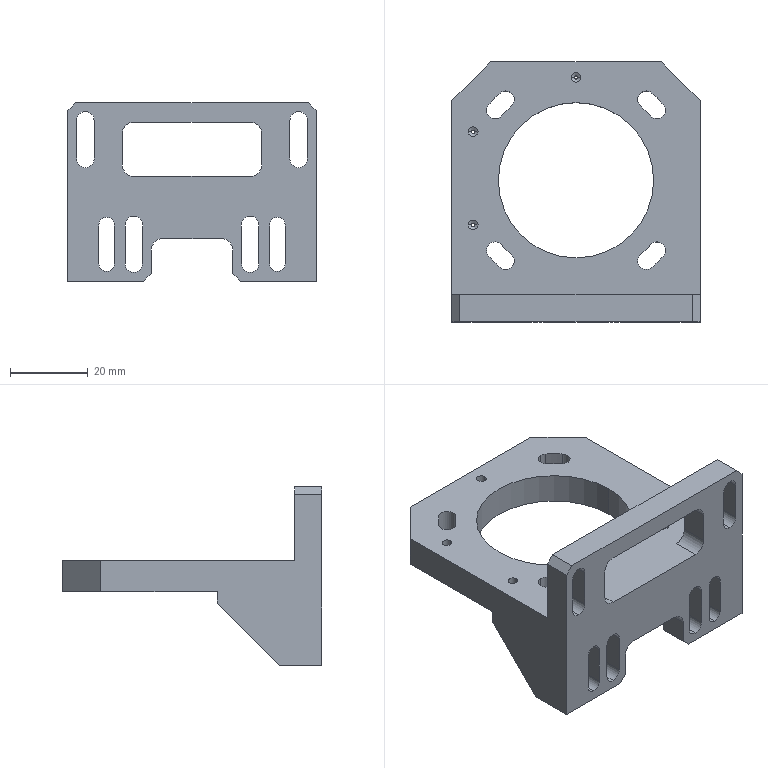NC program | NX | posted with a generic post | part box 64 x 67 x 46 mm
Lines 2506 to 3573 of 8734:
(ZLEVEL_PROFILE_COPY_1_COPY , TOOL : D3)
N4998 T03 M6
N5000 G54
N5002 G17 G0 G90 X-28.2 Y-16.714 B0. C0. S5500 M3
N5004 G43 Z30. H3
N5006 Z0.8
N5008 G94 G1 Y-18.565 Z0.703 F1000.
N5010 X-28.166 Y-18.746 Z0.693
N5012 X-28.017 Y-18.987 Z0.678
N5014 X-27.785 Y-19.15 Z0.664
N5016 X-27.509 Y-19.21 Z0.649
N5018 X-27.231 Y-19.157 Z0.634
N5020 X-27.029 Y-19.031 Z0.622
N5022 X-26.879 Y-18.845 Z0.609
N5024 X-26.8 Y-18.619 Z0.596
N5026 Y-8.381 Z0.06
N5028 X-26.907 Y-8.109 Z0.045
N5030 X-27.115 Y-7.903 Z0.029
N5032 X-27.389 Y-7.799 Z0.014
N5034 X-27.626 Y-7.801 Z0.001
N5036 X-27.893 Y-7.909 Z-0.014
N5038 X-28.095 Y-8.113 Z-0.029
N5040 X-28.2 Y-8.381 Z-0.044
N5042 Y-8.5 Z-0.05
N5044 Y-18.5 F1250.
N5046 G3 X-27.5 Y-19.2 R0.7
N5048 X-26.8 Y-18.5 R0.7
N5050 G1 Y-8.5
N5052 G3 X-27.5 Y-7.8 R0.7
N5054 X-28.2 Y-8.5 R0.7
N5056 G1 Y-11.364 Z-0.1
N5058 Y-18.5
N5060 G3 X-27.5 Y-19.2 R0.7
N5062 X-26.8 Y-18.5 R0.7
N5064 G1 Y-8.5
N5066 G3 X-27.5 Y-7.8 R0.7
N5068 X-28.2 Y-8.5 R0.7
N5070 G1 Y-11.364 Z-0.15
N5072 Y-18.5
N5074 G3 X-27.5 Y-19.2 R0.7
N5076 X-26.8 Y-18.5 R0.7
N5078 G1 Y-8.5
N5080 G3 X-27.5 Y-7.8 R0.7
N5082 X-28.2 Y-8.5 R0.7
N5084 G1 Y-11.364 Z-0.2
N5086 Y-18.5
N5088 G3 X-27.5 Y-19.2 R0.7
N5090 X-26.8 Y-18.5 R0.7
N5092 G1 Y-8.5
N5094 G3 X-27.5 Y-7.8 R0.7
N5096 X-28.2 Y-8.5 R0.7
N5098 G1 Y-11.364 Z-0.25
N5100 Y-18.5
N5102 G3 X-27.5 Y-19.2 R0.7
N5104 X-26.8 Y-18.5 R0.7
N5106 G1 Y-8.5
N5108 G3 X-27.5 Y-7.8 R0.7
N5110 X-28.2 Y-8.5 R0.7
N5112 G1 Y-11.364 Z-0.3
N5114 Y-18.5
N5116 G3 X-27.5 Y-19.2 R0.7
N5118 X-26.8 Y-18.5 R0.7
N5120 G1 Y-8.5
N5122 G3 X-27.5 Y-7.8 R0.7
N5124 X-28.2 Y-8.5 R0.7
N5126 G1 Y-11.364 Z-0.35
N5128 Y-18.5
N5130 G3 X-27.5 Y-19.2 R0.7
N5132 X-26.8 Y-18.5 R0.7
N5134 G1 Y-8.5
N5136 G3 X-27.5 Y-7.8 R0.7
N5138 X-28.2 Y-8.5 R0.7
N5140 G1 Y-11.364 Z-0.4
N5142 Y-18.5
N5144 G3 X-27.5 Y-19.2 R0.7
N5146 X-26.8 Y-18.5 R0.7
N5148 G1 Y-8.5
N5150 G3 X-27.5 Y-7.8 R0.7
N5152 X-28.2 Y-8.5 R0.7
N5154 G1 Y-11.364 Z-0.45
N5156 Y-18.5
N5158 G3 X-27.5 Y-19.2 R0.7
N5160 X-26.8 Y-18.5 R0.7
N5162 G1 Y-8.5
N5164 G3 X-27.5 Y-7.8 R0.7
N5166 X-28.2 Y-8.5 R0.7
N5168 G1 Y-11.364 Z-0.5
N5170 Y-18.5
N5172 G3 X-27.5 Y-19.2 R0.7
N5174 X-26.8 Y-18.5 R0.7
N5176 G1 Y-8.5
N5178 G3 X-27.5 Y-7.8 R0.7
N5180 X-28.2 Y-8.5 R0.7
N5182 G1 Y-11.364 Z-0.55
N5184 Y-18.5
N5186 G3 X-27.5 Y-19.2 R0.7
N5188 X-26.8 Y-18.5 R0.7
N5190 G1 Y-8.5
N5192 G3 X-27.5 Y-7.8 R0.7
N5194 X-28.2 Y-8.5 R0.7
N5196 G1 Y-11.364 Z-0.6
N5198 Y-18.5
N5200 G3 X-27.5 Y-19.2 R0.7
N5202 X-26.8 Y-18.5 R0.7
N5204 G1 Y-8.5
N5206 G3 X-27.5 Y-7.8 R0.7
N5208 X-28.2 Y-8.5 R0.7
N5210 G1 Y-11.364 Z-0.65
N5212 Y-18.5
N5214 G3 X-27.5 Y-19.2 R0.7
N5216 X-26.8 Y-18.5 R0.7
N5218 G1 Y-8.5
N5220 G3 X-27.5 Y-7.8 R0.7
N5222 X-28.2 Y-8.5 R0.7
N5224 G1 Y-11.364 Z-0.7
N5226 Y-18.5
N5228 G3 X-27.5 Y-19.2 R0.7
N5230 X-26.8 Y-18.5 R0.7
N5232 G1 Y-8.5
N5234 G3 X-27.5 Y-7.8 R0.7
N5236 X-28.2 Y-8.5 R0.7
N5238 G1 Y-11.364 Z-0.75
N5240 Y-18.5
N5242 G3 X-27.5 Y-19.2 R0.7
N5244 X-26.8 Y-18.5 R0.7
N5246 G1 Y-8.5
N5248 G3 X-27.5 Y-7.8 R0.7
N5250 X-28.2 Y-8.5 R0.7
N5252 G1 Y-11.364 Z-0.8
N5254 Y-18.5
N5256 G3 X-27.5 Y-19.2 R0.7
N5258 X-26.8 Y-18.5 R0.7
N5260 G1 Y-8.5
N5262 G3 X-27.5 Y-7.8 R0.7
N5264 X-28.2 Y-8.5 R0.7
N5266 G1 Y-11.364 Z-0.85
N5268 Y-18.5
N5270 G3 X-27.5 Y-19.2 R0.7
N5272 X-26.8 Y-18.5 R0.7
N5274 G1 Y-8.5
N5276 G3 X-27.5 Y-7.8 R0.7
N5278 X-28.2 Y-8.5 R0.7
N5280 G1 Y-11.364 Z-0.9
N5282 Y-18.5
N5284 G3 X-27.5 Y-19.2 R0.7
N5286 X-26.8 Y-18.5 R0.7
N5288 G1 Y-8.5
N5290 G3 X-27.5 Y-7.8 R0.7
N5292 X-28.2 Y-8.5 R0.7
N5294 G1 Y-11.364 Z-0.95
N5296 Y-18.5
N5298 G3 X-27.5 Y-19.2 R0.7
N5300 X-26.8 Y-18.5 R0.7
N5302 G1 Y-8.5
N5304 G3 X-27.5 Y-7.8 R0.7
N5306 X-28.2 Y-8.5 R0.7
N5308 G1 Y-11.364 Z-1.
N5310 Y-18.5
N5312 G3 X-27.5 Y-19.2 R0.7
N5314 X-26.8 Y-18.5 R0.7
N5316 G1 Y-8.5
N5318 G3 X-27.5 Y-7.8 R0.7
N5320 X-28.2 Y-8.5 R0.7
N5322 G1 Y-11.364 Z-1.05
N5324 Y-18.5
N5326 G3 X-27.5 Y-19.2 R0.7
N5328 X-26.8 Y-18.5 R0.7
N5330 G1 Y-8.5
N5332 G3 X-27.5 Y-7.8 R0.7
N5334 X-28.2 Y-8.5 R0.7
N5336 G1 Y-11.364 Z-1.1
N5338 Y-18.5
N5340 G3 X-27.5 Y-19.2 R0.7
N5342 X-26.8 Y-18.5 R0.7
N5344 G1 Y-8.5
N5346 G3 X-27.5 Y-7.8 R0.7
N5348 X-28.2 Y-8.5 R0.7
N5350 G1 Y-11.364 Z-1.15
N5352 Y-18.5
N5354 G3 X-27.5 Y-19.2 R0.7
N5356 X-26.8 Y-18.5 R0.7
N5358 G1 Y-8.5
N5360 G3 X-27.5 Y-7.8 R0.7
N5362 X-28.2 Y-8.5 R0.7
N5364 G1 Y-11.364 Z-1.2
N5366 Y-18.5
N5368 G3 X-27.5 Y-19.2 R0.7
N5370 X-26.8 Y-18.5 R0.7
N5372 G1 Y-8.5
N5374 G3 X-27.5 Y-7.8 R0.7
N5376 X-28.2 Y-8.5 R0.7
N5378 G1 Y-11.364 Z-1.25
N5380 Y-18.5
N5382 G3 X-27.5 Y-19.2 R0.7
N5384 X-26.8 Y-18.5 R0.7
N5386 G1 Y-8.5
N5388 G3 X-27.5 Y-7.8 R0.7
N5390 X-28.2 Y-8.5 R0.7
N5392 G1 Y-11.364 Z-1.3
N5394 Y-18.5
N5396 G3 X-27.5 Y-19.2 R0.7
N5398 X-26.8 Y-18.5 R0.7
N5400 G1 Y-8.5
N5402 G3 X-27.5 Y-7.8 R0.7
N5404 X-28.2 Y-8.5 R0.7
N5406 G1 Y-11.364 Z-1.35
N5408 Y-18.5
N5410 G3 X-27.5 Y-19.2 R0.7
N5412 X-26.8 Y-18.5 R0.7
N5414 G1 Y-8.5
N5416 G3 X-27.5 Y-7.8 R0.7
N5418 X-28.2 Y-8.5 R0.7
N5420 G1 Y-11.364 Z-1.4
N5422 Y-18.5
N5424 G3 X-27.5 Y-19.2 R0.7
N5426 X-26.8 Y-18.5 R0.7
N5428 G1 Y-8.5
N5430 G3 X-27.5 Y-7.8 R0.7
N5432 X-28.2 Y-8.5 R0.7
N5434 G1 Y-11.364 Z-1.45
N5436 Y-18.5
N5438 G3 X-27.5 Y-19.2 R0.7
N5440 X-26.8 Y-18.5 R0.7
N5442 G1 Y-8.5
N5444 G3 X-27.5 Y-7.8 R0.7
N5446 X-28.2 Y-8.5 R0.7
N5448 G1 Y-11.364 Z-1.5
N5450 Y-18.5
N5452 G3 X-27.5 Y-19.2 R0.7
N5454 X-26.8 Y-18.5 R0.7
N5456 G1 Y-8.5
N5458 G3 X-27.5 Y-7.8 R0.7
N5460 X-28.2 Y-8.5 R0.7
N5462 G1 Y-11.364 Z-1.55
N5464 Y-18.5
N5466 G3 X-27.5 Y-19.2 R0.7
N5468 X-26.8 Y-18.5 R0.7
N5470 G1 Y-8.5
N5472 G3 X-27.5 Y-7.8 R0.7
N5474 X-28.2 Y-8.5 R0.7
N5476 G1 Y-11.364 Z-1.6
N5478 Y-18.5
N5480 G3 X-27.5 Y-19.2 R0.7
N5482 X-26.8 Y-18.5 R0.7
N5484 G1 Y-8.5
N5486 G3 X-27.5 Y-7.8 R0.7
N5488 X-28.2 Y-8.5 R0.7
N5490 G1 Y-11.364 Z-1.65
N5492 Y-18.5
N5494 G3 X-27.5 Y-19.2 R0.7
N5496 X-26.8 Y-18.5 R0.7
N5498 G1 Y-8.5
N5500 G3 X-27.5 Y-7.8 R0.7
N5502 X-28.2 Y-8.5 R0.7
N5504 G1 Y-11.364 Z-1.7
N5506 Y-18.5
N5508 G3 X-27.5 Y-19.2 R0.7
N5510 X-26.8 Y-18.5 R0.7
N5512 G1 Y-8.5
N5514 G3 X-27.5 Y-7.8 R0.7
N5516 X-28.2 Y-8.5 R0.7
N5518 G1 Y-11.364 Z-1.75
N5520 Y-18.5
N5522 G3 X-27.5 Y-19.2 R0.7
N5524 X-26.8 Y-18.5 R0.7
N5526 G1 Y-8.5
N5528 G3 X-27.5 Y-7.8 R0.7
N5530 X-28.2 Y-8.5 R0.7
N5532 G1 Y-11.364 Z-1.8
N5534 Y-18.5
N5536 G3 X-27.5 Y-19.2 R0.7
N5538 X-26.8 Y-18.5 R0.7
N5540 G1 Y-8.5
N5542 G3 X-27.5 Y-7.8 R0.7
N5544 X-28.2 Y-8.5 R0.7
N5546 G1 Y-11.364 Z-1.85
N5548 Y-18.5
N5550 G3 X-27.5 Y-19.2 R0.7
N5552 X-26.8 Y-18.5 R0.7
N5554 G1 Y-8.5
N5556 G3 X-27.5 Y-7.8 R0.7
N5558 X-28.2 Y-8.5 R0.7
N5560 G1 Y-11.364 Z-1.9
N5562 Y-18.5
N5564 G3 X-27.5 Y-19.2 R0.7
N5566 X-26.8 Y-18.5 R0.7
N5568 G1 Y-8.5
N5570 G3 X-27.5 Y-7.8 R0.7
N5572 X-28.2 Y-8.5 R0.7
N5574 G1 Y-11.364 Z-1.95
N5576 Y-18.5
N5578 G3 X-27.5 Y-19.2 R0.7
N5580 X-26.8 Y-18.5 R0.7
N5582 G1 Y-8.5
N5584 G3 X-27.5 Y-7.8 R0.7
N5586 X-28.2 Y-8.5 R0.7
N5588 G1 Y-11.364 Z-2.
N5590 Y-18.5
N5592 G3 X-27.5 Y-19.2 R0.7
N5594 X-26.8 Y-18.5 R0.7
N5596 G1 Y-8.5
N5598 G3 X-27.5 Y-7.8 R0.7
N5600 X-28.2 Y-8.5 R0.7
N5602 G1 Y-11.364 Z-2.05
N5604 Y-18.5
N5606 G3 X-27.5 Y-19.2 R0.7
N5608 X-26.8 Y-18.5 R0.7
N5610 G1 Y-8.5
N5612 G3 X-27.5 Y-7.8 R0.7
N5614 X-28.2 Y-8.5 R0.7
N5616 G1 Y-11.364 Z-2.1
N5618 Y-18.5
N5620 G3 X-27.5 Y-19.2 R0.7
N5622 X-26.8 Y-18.5 R0.7
N5624 G1 Y-8.5
N5626 G3 X-27.5 Y-7.8 R0.7
N5628 X-28.2 Y-8.5 R0.7
N5630 G1 Y-11.364 Z-2.15
N5632 Y-18.5
N5634 G3 X-27.5 Y-19.2 R0.7
N5636 X-26.8 Y-18.5 R0.7
N5638 G1 Y-8.5
N5640 G3 X-27.5 Y-7.8 R0.7
N5642 X-28.2 Y-8.5 R0.7
N5644 G1 Y-11.364 Z-2.2
N5646 Y-18.5
N5648 G3 X-27.5 Y-19.2 R0.7
N5650 X-26.8 Y-18.5 R0.7
N5652 G1 Y-8.5
N5654 G3 X-27.5 Y-7.8 R0.7
N5656 X-28.2 Y-8.5 R0.7
N5658 G1 Y-11.364 Z-2.25
N5660 Y-18.5
N5662 G3 X-27.5 Y-19.2 R0.7
N5664 X-26.8 Y-18.5 R0.7
N5666 G1 Y-8.5
N5668 G3 X-27.5 Y-7.8 R0.7
N5670 X-28.2 Y-8.5 R0.7
N5672 G1 Y-11.364 Z-2.3
N5674 Y-18.5
N5676 G3 X-27.5 Y-19.2 R0.7
N5678 X-26.8 Y-18.5 R0.7
N5680 G1 Y-8.5
N5682 G3 X-27.5 Y-7.8 R0.7
N5684 X-28.2 Y-8.5 R0.7
N5686 G1 Y-11.364 Z-2.35
N5688 Y-18.5
N5690 G3 X-27.5 Y-19.2 R0.7
N5692 X-26.8 Y-18.5 R0.7
N5694 G1 Y-8.5
N5696 G3 X-27.5 Y-7.8 R0.7
N5698 X-28.2 Y-8.5 R0.7
N5700 G1 Y-11.364 Z-2.4
N5702 Y-18.5
N5704 G3 X-27.5 Y-19.2 R0.7
N5706 X-26.8 Y-18.5 R0.7
N5708 G1 Y-8.5
N5710 G3 X-27.5 Y-7.8 R0.7
N5712 X-28.2 Y-8.5 R0.7
N5714 G1 Y-11.364 Z-2.45
N5716 Y-18.5
N5718 G3 X-27.5 Y-19.2 R0.7
N5720 X-26.8 Y-18.5 R0.7
N5722 G1 Y-8.5
N5724 G3 X-27.5 Y-7.8 R0.7
N5726 X-28.2 Y-8.5 R0.7
N5728 G1 Y-11.364 Z-2.5
N5730 Y-18.5
N5732 G3 X-27.5 Y-19.2 R0.7
N5734 X-26.8 Y-18.5 R0.7
N5736 G1 Y-8.5
N5738 G3 X-27.5 Y-7.8 R0.7
N5740 X-28.2 Y-8.5 R0.7
N5742 G1 Y-11.364 Z-2.55
N5744 Y-18.5
N5746 G3 X-27.5 Y-19.2 R0.7
N5748 X-26.8 Y-18.5 R0.7
N5750 G1 Y-8.5
N5752 G3 X-27.5 Y-7.8 R0.7
N5754 X-28.2 Y-8.5 R0.7
N5756 G1 Y-11.364 Z-2.6
N5758 Y-18.5
N5760 G3 X-27.5 Y-19.2 R0.7
N5762 X-26.8 Y-18.5 R0.7
N5764 G1 Y-8.5
N5766 G3 X-27.5 Y-7.8 R0.7
N5768 X-28.2 Y-8.5 R0.7
N5770 G1 Y-11.364 Z-2.65
N5772 Y-18.5
N5774 G3 X-27.5 Y-19.2 R0.7
N5776 X-26.8 Y-18.5 R0.7
N5778 G1 Y-8.5
N5780 G3 X-27.5 Y-7.8 R0.7
N5782 X-28.2 Y-8.5 R0.7
N5784 G1 Y-11.364 Z-2.7
N5786 Y-18.5
N5788 G3 X-27.5 Y-19.2 R0.7
N5790 X-26.8 Y-18.5 R0.7
N5792 G1 Y-8.5
N5794 G3 X-27.5 Y-7.8 R0.7
N5796 X-28.2 Y-8.5 R0.7
N5798 G1 Y-11.364 Z-2.75
N5800 Y-18.5
N5802 G3 X-27.5 Y-19.2 R0.7
N5804 X-26.8 Y-18.5 R0.7
N5806 G1 Y-8.5
N5808 G3 X-27.5 Y-7.8 R0.7
N5810 X-28.2 Y-8.5 R0.7
N5812 G1 Y-11.364 Z-2.8
N5814 Y-18.5
N5816 G3 X-27.5 Y-19.2 R0.7
N5818 X-26.8 Y-18.5 R0.7
N5820 G1 Y-8.5
N5822 G3 X-27.5 Y-7.8 R0.7
N5824 X-28.2 Y-8.5 R0.7
N5826 G1 Y-11.364 Z-2.85
N5828 Y-18.5
N5830 G3 X-27.5 Y-19.2 R0.7
N5832 X-26.8 Y-18.5 R0.7
N5834 G1 Y-8.5
N5836 G3 X-27.5 Y-7.8 R0.7
N5838 X-28.2 Y-8.5 R0.7
N5840 G1 Y-11.364 Z-2.9
N5842 Y-18.5
N5844 G3 X-27.5 Y-19.2 R0.7
N5846 X-26.8 Y-18.5 R0.7
N5848 G1 Y-8.5
N5850 G3 X-27.5 Y-7.8 R0.7
N5852 X-28.2 Y-8.5 R0.7
N5854 G1 Y-11.364 Z-2.95
N5856 Y-18.5
N5858 G3 X-27.5 Y-19.2 R0.7
N5860 X-26.8 Y-18.5 R0.7
N5862 G1 Y-8.5
N5864 G3 X-27.5 Y-7.8 R0.7
N5866 X-28.2 Y-8.5 R0.7
N5868 G1 Y-11.364 Z-3.
N5870 Y-18.5
N5872 G3 X-27.5 Y-19.2 R0.7
N5874 X-26.8 Y-18.5 R0.7
N5876 G1 Y-8.5
N5878 G3 X-27.5 Y-7.8 R0.7
N5880 X-28.2 Y-8.5 R0.7
N5882 G1 Y-11.364 Z-3.05
N5884 Y-18.5
N5886 G3 X-27.5 Y-19.2 R0.7
N5888 X-26.8 Y-18.5 R0.7
N5890 G1 Y-8.5
N5892 G3 X-27.5 Y-7.8 R0.7
N5894 X-28.2 Y-8.5 R0.7
N5896 G1 Y-11.364 Z-3.1
N5898 Y-18.5
N5900 G3 X-27.5 Y-19.2 R0.7
N5902 X-26.8 Y-18.5 R0.7
N5904 G1 Y-8.5
N5906 G3 X-27.5 Y-7.8 R0.7
N5908 X-28.2 Y-8.5 R0.7
N5910 G1 Y-11.364 Z-3.15
N5912 Y-18.5
N5914 G3 X-27.5 Y-19.2 R0.7
N5916 X-26.8 Y-18.5 R0.7
N5918 G1 Y-8.5
N5920 G3 X-27.5 Y-7.8 R0.7
N5922 X-28.2 Y-8.5 R0.7
N5924 G1 Y-11.364 Z-3.2
N5926 Y-18.5
N5928 G3 X-27.5 Y-19.2 R0.7
N5930 X-26.8 Y-18.5 R0.7
N5932 G1 Y-8.5
N5934 G3 X-27.5 Y-7.8 R0.7
N5936 X-28.2 Y-8.5 R0.7
N5938 G1 Y-11.364 Z-3.25
N5940 Y-18.5
N5942 G3 X-27.5 Y-19.2 R0.7
N5944 X-26.8 Y-18.5 R0.7
N5946 G1 Y-8.5
N5948 G3 X-27.5 Y-7.8 R0.7
N5950 X-28.2 Y-8.5 R0.7
N5952 G1 Y-11.364 Z-3.3
N5954 Y-18.5
N5956 G3 X-27.5 Y-19.2 R0.7
N5958 X-26.8 Y-18.5 R0.7
N5960 G1 Y-8.5
N5962 G3 X-27.5 Y-7.8 R0.7
N5964 X-28.2 Y-8.5 R0.7
N5966 G1 Y-11.364 Z-3.35
N5968 Y-18.5
N5970 G3 X-27.5 Y-19.2 R0.7
N5972 X-26.8 Y-18.5 R0.7
N5974 G1 Y-8.5
N5976 G3 X-27.5 Y-7.8 R0.7
N5978 X-28.2 Y-8.5 R0.7
N5980 G1 Y-11.364 Z-3.4
N5982 Y-18.5
N5984 G3 X-27.5 Y-19.2 R0.7
N5986 X-26.8 Y-18.5 R0.7
N5988 G1 Y-8.5
N5990 G3 X-27.5 Y-7.8 R0.7
N5992 X-28.2 Y-8.5 R0.7
N5994 G1 Y-11.364 Z-3.45
N5996 Y-18.5
N5998 G3 X-27.5 Y-19.2 R0.7
N6000 X-26.8 Y-18.5 R0.7
N6002 G1 Y-8.5
N6004 G3 X-27.5 Y-7.8 R0.7
N6006 X-28.2 Y-8.5 R0.7
N6008 G1 Y-11.364 Z-3.5
N6010 Y-18.5
N6012 G3 X-27.5 Y-19.2 R0.7
N6014 X-26.8 Y-18.5 R0.7
N6016 G1 Y-8.5
N6018 G3 X-27.5 Y-7.8 R0.7
N6020 X-28.2 Y-8.5 R0.7
N6022 G1 Y-11.364 Z-3.55
N6024 Y-18.5
N6026 G3 X-27.5 Y-19.2 R0.7
N6028 X-26.8 Y-18.5 R0.7
N6030 G1 Y-8.5
N6032 G3 X-27.5 Y-7.8 R0.7
N6034 X-28.2 Y-8.5 R0.7
N6036 G1 Y-11.364 Z-3.6
N6038 Y-18.5
N6040 G3 X-27.5 Y-19.2 R0.7
N6042 X-26.8 Y-18.5 R0.7
N6044 G1 Y-8.5
N6046 G3 X-27.5 Y-7.8 R0.7
N6048 X-28.2 Y-8.5 R0.7
N6050 G1 Y-11.364 Z-3.65
N6052 Y-18.5
N6054 G3 X-27.5 Y-19.2 R0.7
N6056 X-26.8 Y-18.5 R0.7
N6058 G1 Y-8.5
N6060 G3 X-27.5 Y-7.8 R0.7
N6062 X-28.2 Y-8.5 R0.7
N6064 G1 Y-11.364 Z-3.7
N6066 Y-18.5
N6068 G3 X-27.5 Y-19.2 R0.7
N6070 X-26.8 Y-18.5 R0.7
N6072 G1 Y-8.5
N6074 G3 X-27.5 Y-7.8 R0.7
N6076 X-28.2 Y-8.5 R0.7
N6078 G1 Y-11.364 Z-3.75
N6080 Y-18.5
N6082 G3 X-27.5 Y-19.2 R0.7
N6084 X-26.8 Y-18.5 R0.7
N6086 G1 Y-8.5
N6088 G3 X-27.5 Y-7.8 R0.7
N6090 X-28.2 Y-8.5 R0.7
N6092 G1 Y-11.364 Z-3.8
N6094 Y-18.5
N6096 G3 X-27.5 Y-19.2 R0.7
N6098 X-26.8 Y-18.5 R0.7
N6100 G1 Y-8.5
N6102 G3 X-27.5 Y-7.8 R0.7
N6104 X-28.2 Y-8.5 R0.7
N6106 G1 Y-11.364 Z-3.85
N6108 Y-18.5
N6110 G3 X-27.5 Y-19.2 R0.7
N6112 X-26.8 Y-18.5 R0.7
N6114 G1 Y-8.5
N6116 G3 X-27.5 Y-7.8 R0.7
N6118 X-28.2 Y-8.5 R0.7
N6120 G1 Y-11.364 Z-3.9
N6122 Y-18.5
N6124 G3 X-27.5 Y-19.2 R0.7
N6126 X-26.8 Y-18.5 R0.7
N6128 G1 Y-8.5
N6130 G3 X-27.5 Y-7.8 R0.7
N6132 X-28.2 Y-8.5 R0.7
N6134 G1 Y-11.364 Z-3.95
N6136 Y-18.5
N6138 G3 X-27.5 Y-19.2 R0.7
N6140 X-26.8 Y-18.5 R0.7
N6142 G1 Y-8.5
N6144 G3 X-27.5 Y-7.8 R0.7
N6146 X-28.2 Y-8.5 R0.7
N6148 G1 Y-11.364 Z-4.
N6150 Y-18.5
N6152 G3 X-27.5 Y-19.2 R0.7
N6154 X-26.8 Y-18.5 R0.7
N6156 G1 Y-8.5
N6158 G3 X-27.5 Y-7.8 R0.7
N6160 X-28.2 Y-8.5 R0.7
N6162 G1 Y-11.364 Z-4.05
N6164 Y-18.5
N6166 G3 X-27.5 Y-19.2 R0.7
N6168 X-26.8 Y-18.5 R0.7
N6170 G1 Y-8.5
N6172 G3 X-27.5 Y-7.8 R0.7
N6174 X-28.2 Y-8.5 R0.7
N6176 G1 Y-11.364 Z-4.1
N6178 Y-18.5
N6180 G3 X-27.5 Y-19.2 R0.7
N6182 X-26.8 Y-18.5 R0.7
N6184 G1 Y-8.5
N6186 G3 X-27.5 Y-7.8 R0.7
N6188 X-28.2 Y-8.5 R0.7
N6190 G1 Y-11.364 Z-4.15
N6192 Y-18.5
N6194 G3 X-27.5 Y-19.2 R0.7
N6196 X-26.8 Y-18.5 R0.7
N6198 G1 Y-8.5
N6200 G3 X-27.5 Y-7.8 R0.7
N6202 X-28.2 Y-8.5 R0.7
N6204 G1 Y-11.364 Z-4.2
N6206 Y-18.5
N6208 G3 X-27.5 Y-19.2 R0.7
N6210 X-26.8 Y-18.5 R0.7
N6212 G1 Y-8.5
N6214 G3 X-27.5 Y-7.8 R0.7
N6216 X-28.2 Y-8.5 R0.7
N6218 G1 Y-11.364 Z-4.25
N6220 Y-18.5
N6222 G3 X-27.5 Y-19.2 R0.7
N6224 X-26.8 Y-18.5 R0.7
N6226 G1 Y-8.5
N6228 G3 X-27.5 Y-7.8 R0.7
N6230 X-28.2 Y-8.5 R0.7
N6232 G1 Y-11.364 Z-4.3
N6234 Y-18.5
N6236 G3 X-27.5 Y-19.2 R0.7
N6238 X-26.8 Y-18.5 R0.7
N6240 G1 Y-8.5
N6242 G3 X-27.5 Y-7.8 R0.7
N6244 X-28.2 Y-8.5 R0.7
N6246 G1 Y-11.364 Z-4.35
N6248 Y-18.5
N6250 G3 X-27.5 Y-19.2 R0.7
N6252 X-26.8 Y-18.5 R0.7
N6254 G1 Y-8.5
N6256 G3 X-27.5 Y-7.8 R0.7
N6258 X-28.2 Y-8.5 R0.7
N6260 G1 Y-11.364 Z-4.4
N6262 Y-18.5
N6264 G3 X-27.5 Y-19.2 R0.7
N6266 X-26.8 Y-18.5 R0.7
N6268 G1 Y-8.5
N6270 G3 X-27.5 Y-7.8 R0.7
N6272 X-28.2 Y-8.5 R0.7
N6274 G1 Y-11.364 Z-4.45
N6276 Y-18.5
N6278 G3 X-27.5 Y-19.2 R0.7
N6280 X-26.8 Y-18.5 R0.7
N6282 G1 Y-8.5
N6284 G3 X-27.5 Y-7.8 R0.7
N6286 X-28.2 Y-8.5 R0.7
N6288 G1 Y-11.364 Z-4.5
N6290 Y-18.5
N6292 G3 X-27.5 Y-19.2 R0.7
N6294 X-26.8 Y-18.5 R0.7
N6296 G1 Y-8.5
N6298 G3 X-27.5 Y-7.8 R0.7
N6300 X-28.2 Y-8.5 R0.7
N6302 G1 Y-11.364 Z-4.55
N6304 Y-18.5
N6306 G3 X-27.5 Y-19.2 R0.7
N6308 X-26.8 Y-18.5 R0.7
N6310 G1 Y-8.5
N6312 G3 X-27.5 Y-7.8 R0.7
N6314 X-28.2 Y-8.5 R0.7
N6316 G1 Y-11.364 Z-4.6
N6318 Y-18.5
N6320 G3 X-27.5 Y-19.2 R0.7
N6322 X-26.8 Y-18.5 R0.7
N6324 G1 Y-8.5
N6326 G3 X-27.5 Y-7.8 R0.7
N6328 X-28.2 Y-8.5 R0.7
N6330 G1 Y-11.364 Z-4.65
N6332 Y-18.5
N6334 G3 X-27.5 Y-19.2 R0.7
N6336 X-26.8 Y-18.5 R0.7
N6338 G1 Y-8.5
N6340 G3 X-27.5 Y-7.8 R0.7
N6342 X-28.2 Y-8.5 R0.7
N6344 G1 Y-11.364 Z-4.7
N6346 Y-18.5
N6348 G3 X-27.5 Y-19.2 R0.7
N6350 X-26.8 Y-18.5 R0.7
N6352 G1 Y-8.5
N6354 G3 X-27.5 Y-7.8 R0.7
N6356 X-28.2 Y-8.5 R0.7
N6358 G1 Y-11.364 Z-4.75
N6360 Y-18.5
N6362 G3 X-27.5 Y-19.2 R0.7
N6364 X-26.8 Y-18.5 R0.7
N6366 G1 Y-8.5
N6368 G3 X-27.5 Y-7.8 R0.7
N6370 X-28.2 Y-8.5 R0.7
N6372 G1 Y-11.364 Z-4.8
N6374 Y-18.5
N6376 G3 X-27.5 Y-19.2 R0.7
N6378 X-26.8 Y-18.5 R0.7
N6380 G1 Y-8.5
N6382 G3 X-27.5 Y-7.8 R0.7
N6384 X-28.2 Y-8.5 R0.7
N6386 G1 Y-11.364 Z-4.85
N6388 Y-18.5
N6390 G3 X-27.5 Y-19.2 R0.7
N6392 X-26.8 Y-18.5 R0.7
N6394 G1 Y-8.5
N6396 G3 X-27.5 Y-7.8 R0.7
N6398 X-28.2 Y-8.5 R0.7
N6400 G1 Y-11.364 Z-4.9
N6402 Y-18.5
N6404 G3 X-27.5 Y-19.2 R0.7
N6406 X-26.8 Y-18.5 R0.7
N6408 G1 Y-8.5
N6410 G3 X-27.5 Y-7.8 R0.7
N6412 X-28.2 Y-8.5 R0.7
N6414 G1 Y-11.364 Z-4.95
N6416 Y-18.5
N6418 G3 X-27.5 Y-19.2 R0.7
N6420 X-26.8 Y-18.5 R0.7
N6422 G1 Y-8.5
N6424 G3 X-27.5 Y-7.8 R0.7
N6426 X-28.2 Y-8.5 R0.7
N6428 G1 Y-11.364 Z-5.
N6430 Y-18.5
N6432 G3 X-27.5 Y-19.2 R0.7
N6434 X-26.8 Y-18.5 R0.7
N6436 G1 Y-8.5
N6438 G3 X-27.5 Y-7.8 R0.7
N6440 X-28.2 Y-8.5 R0.7
N6442 G1 Y-11.364 Z-5.05
N6444 Y-18.5
N6446 G3 X-27.5 Y-19.2 R0.7
N6448 X-26.8 Y-18.5 R0.7
N6450 G1 Y-8.5
N6452 G3 X-27.5 Y-7.8 R0.7
N6454 X-28.2 Y-8.5 R0.7
N6456 G1 Y-11.364 Z-5.1
N6458 Y-18.5
N6460 G3 X-27.5 Y-19.2 R0.7
N6462 X-26.8 Y-18.5 R0.7
N6464 G1 Y-8.5
N6466 G3 X-27.5 Y-7.8 R0.7
N6468 X-28.2 Y-8.5 R0.7
N6470 G1 Y-11.364 Z-5.15
N6472 Y-18.5
N6474 G3 X-27.5 Y-19.2 R0.7
N6476 X-26.8 Y-18.5 R0.7
N6478 G1 Y-8.5
N6480 G3 X-27.5 Y-7.8 R0.7
N6482 X-28.2 Y-8.5 R0.7
N6484 G1 Y-11.364 Z-5.2
N6486 Y-18.5
N6488 G3 X-27.5 Y-19.2 R0.7
N6490 X-26.8 Y-18.5 R0.7
N6492 G1 Y-8.5
N6494 G3 X-27.5 Y-7.8 R0.7
N6496 X-28.2 Y-8.5 R0.7
N6498 G1 Y-11.364 Z-5.25
N6500 Y-18.5
N6502 G3 X-27.5 Y-19.2 R0.7
N6504 X-26.8 Y-18.5 R0.7
N6506 G1 Y-8.5
N6508 G3 X-27.5 Y-7.8 R0.7
N6510 X-28.2 Y-8.5 R0.7
N6512 G1 Y-11.364 Z-5.3
N6514 Y-18.5
N6516 G3 X-27.5 Y-19.2 R0.7
N6518 X-26.8 Y-18.5 R0.7
N6520 G1 Y-8.5
N6522 G3 X-27.5 Y-7.8 R0.7
N6524 X-28.2 Y-8.5 R0.7
N6526 G1 Y-11.364 Z-5.35
N6528 Y-18.5
N6530 G3 X-27.5 Y-19.2 R0.7
N6532 X-26.8 Y-18.5 R0.7
N6534 G1 Y-8.5
N6536 G3 X-27.5 Y-7.8 R0.7
N6538 X-28.2 Y-8.5 R0.7
N6540 G1 Y-11.364 Z-5.4
N6542 Y-18.5
N6544 G3 X-27.5 Y-19.2 R0.7
N6546 X-26.8 Y-18.5 R0.7
N6548 G1 Y-8.5
N6550 G3 X-27.5 Y-7.8 R0.7
N6552 X-28.2 Y-8.5 R0.7
N6554 G1 Y-11.364 Z-5.45
N6556 Y-18.5
N6558 G3 X-27.5 Y-19.2 R0.7
N6560 X-26.8 Y-18.5 R0.7
N6562 G1 Y-8.5
N6564 G3 X-27.5 Y-7.8 R0.7
N6566 X-28.2 Y-8.5 R0.7
N6568 G1 Y-11.364 Z-5.5
N6570 Y-18.5
N6572 G3 X-27.5 Y-19.2 R0.7
N6574 X-26.8 Y-18.5 R0.7
N6576 G1 Y-8.5
N6578 G3 X-27.5 Y-7.8 R0.7
N6580 X-28.2 Y-8.5 R0.7
N6582 G1 Y-11.364 Z-5.55
N6584 Y-18.5
N6586 G3 X-27.5 Y-19.2 R0.7
N6588 X-26.8 Y-18.5 R0.7
N6590 G1 Y-8.5
N6592 G3 X-27.5 Y-7.8 R0.7
N6594 X-28.2 Y-8.5 R0.7
N6596 G1 Y-11.364 Z-5.6
N6598 Y-18.5
N6600 G3 X-27.5 Y-19.2 R0.7
N6602 X-26.8 Y-18.5 R0.7
N6604 G1 Y-8.5
N6606 G3 X-27.5 Y-7.8 R0.7
N6608 X-28.2 Y-8.5 R0.7
N6610 G1 Y-11.364 Z-5.65
N6612 Y-18.5
N6614 G3 X-27.5 Y-19.2 R0.7
N6616 X-26.8 Y-18.5 R0.7
N6618 G1 Y-8.5
N6620 G3 X-27.5 Y-7.8 R0.7
N6622 X-28.2 Y-8.5 R0.7
N6624 G1 Y-11.364 Z-5.7
N6626 Y-18.5
N6628 G3 X-27.5 Y-19.2 R0.7
N6630 X-26.8 Y-18.5 R0.7
N6632 G1 Y-8.5
N6634 G3 X-27.5 Y-7.8 R0.7
N6636 X-28.2 Y-8.5 R0.7
N6638 G1 Y-11.364 Z-5.75
N6640 Y-18.5
N6642 G3 X-27.5 Y-19.2 R0.7
N6644 X-26.8 Y-18.5 R0.7
N6646 G1 Y-8.5
N6648 G3 X-27.5 Y-7.8 R0.7
N6650 X-28.2 Y-8.5 R0.7
N6652 G1 Y-11.364 Z-5.8
N6654 Y-18.5
N6656 G3 X-27.5 Y-19.2 R0.7
N6658 X-26.8 Y-18.5 R0.7
N6660 G1 Y-8.5
N6662 G3 X-27.5 Y-7.8 R0.7
N6664 X-28.2 Y-8.5 R0.7
N6666 G1 Y-11.364 Z-5.85
N6668 Y-18.5
N6670 G3 X-27.5 Y-19.2 R0.7
N6672 X-26.8 Y-18.5 R0.7
N6674 G1 Y-8.5
N6676 G3 X-27.5 Y-7.8 R0.7
N6678 X-28.2 Y-8.5 R0.7
N6680 G1 Y-11.364 Z-5.9
N6682 Y-18.5
N6684 G3 X-27.5 Y-19.2 R0.7
N6686 X-26.8 Y-18.5 R0.7
N6688 G1 Y-8.5
N6690 G3 X-27.5 Y-7.8 R0.7
N6692 X-28.2 Y-8.5 R0.7
N6694 G1 Y-11.364 Z-5.95
N6696 Y-18.5
N6698 G3 X-27.5 Y-19.2 R0.7
N6700 X-26.8 Y-18.5 R0.7
N6702 G1 Y-8.5
N6704 G3 X-27.5 Y-7.8 R0.7
N6706 X-28.2 Y-8.5 R0.7
N6708 G1 Y-11.364 Z-6.
N6710 Y-18.5
N6712 G3 X-27.5 Y-19.2 R0.7
N6714 X-26.8 Y-18.5 R0.7
N6716 G1 Y-8.5
N6718 G3 X-27.5 Y-7.8 R0.7
N6720 X-28.2 Y-8.5 R0.7
N6722 G1 Y-11.364 Z-6.05
N6724 Y-18.5
N6726 G3 X-27.5 Y-19.2 R0.7
N6728 X-26.8 Y-18.5 R0.7
N6730 G1 Y-8.5
N6732 G3 X-27.5 Y-7.8 R0.7
N6734 X-28.2 Y-8.5 R0.7
N6736 G1 Y-11.364 Z-6.1
N6738 Y-18.5
N6740 G3 X-27.5 Y-19.2 R0.7
N6742 X-26.8 Y-18.5 R0.7
N6744 G1 Y-8.5
N6746 G3 X-27.5 Y-7.8 R0.7
N6748 X-28.2 Y-8.5 R0.7
N6750 G1 Y-11.364 Z-6.15
N6752 Y-18.5
N6754 G3 X-27.5 Y-19.2 R0.7
N6756 X-26.8 Y-18.5 R0.7
N6758 G1 Y-8.5
N6760 G3 X-27.5 Y-7.8 R0.7
N6762 X-28.2 Y-8.5 R0.7
N6764 G1 Y-11.364 Z-6.2
N6766 Y-18.5
N6768 G3 X-27.5 Y-19.2 R0.7
N6770 X-26.8 Y-18.5 R0.7
N6772 G1 Y-8.5
N6774 G3 X-27.5 Y-7.8 R0.7
N6776 X-28.2 Y-8.5 R0.7
N6778 G1 Y-11.364 Z-6.25
N6780 Y-18.5
N6782 G3 X-27.5 Y-19.2 R0.7
N6784 X-26.8 Y-18.5 R0.7
N6786 G1 Y-8.5
N6788 G3 X-27.5 Y-7.8 R0.7
N6790 X-28.2 Y-8.5 R0.7
N6792 G1 Y-11.364 Z-6.3
N6794 Y-18.5
N6796 G3 X-27.5 Y-19.2 R0.7
N6798 X-26.8 Y-18.5 R0.7
N6800 G1 Y-8.5
N6802 G3 X-27.5 Y-7.8 R0.7
N6804 X-28.2 Y-8.5 R0.7
N6806 G1 Y-11.364 Z-6.35
N6808 Y-18.5
N6810 G3 X-27.5 Y-19.2 R0.7
N6812 X-26.8 Y-18.5 R0.7
N6814 G1 Y-8.5
N6816 G3 X-27.5 Y-7.8 R0.7
N6818 X-28.2 Y-8.5 R0.7
N6820 G1 Y-11.364 Z-6.4
N6822 Y-18.5
N6824 G3 X-27.5 Y-19.2 R0.7
N6826 X-26.8 Y-18.5 R0.7
N6828 G1 Y-8.5
N6830 G3 X-27.5 Y-7.8 R0.7
N6832 X-28.2 Y-8.5 R0.7
N6834 G1 Y-11.364 Z-6.45
N6836 Y-18.5
N6838 G3 X-27.5 Y-19.2 R0.7
N6840 X-26.8 Y-18.5 R0.7
N6842 G1 Y-8.5
N6844 G3 X-27.5 Y-7.8 R0.7
N6846 X-28.2 Y-8.5 R0.7
N6848 G1 Y-11.364 Z-6.5
N6850 Y-18.5
N6852 G3 X-27.5 Y-19.2 R0.7
N6854 X-26.8 Y-18.5 R0.7
N6856 G1 Y-8.5
N6858 G3 X-27.5 Y-7.8 R0.7
N6860 X-28.2 Y-8.5 R0.7
N6862 G1 Y-11.364 Z-6.55
N6864 Y-18.5
N6866 G3 X-27.5 Y-19.2 R0.7
N6868 X-26.8 Y-18.5 R0.7
N6870 G1 Y-8.5
N6872 G3 X-27.5 Y-7.8 R0.7
N6874 X-28.2 Y-8.5 R0.7
N6876 G1 Y-11.364 Z-6.6
N6878 Y-18.5
N6880 G3 X-27.5 Y-19.2 R0.7
N6882 X-26.8 Y-18.5 R0.7
N6884 G1 Y-8.5
N6886 G3 X-27.5 Y-7.8 R0.7
N6888 X-28.2 Y-8.5 R0.7
N6890 G1 Y-11.364 Z-6.65
N6892 Y-18.5
N6894 G3 X-27.5 Y-19.2 R0.7
N6896 X-26.8 Y-18.5 R0.7
N6898 G1 Y-8.5
N6900 G3 X-27.5 Y-7.8 R0.7
N6902 X-28.2 Y-8.5 R0.7
N6904 G1 Y-11.364 Z-6.7
N6906 Y-18.5
N6908 G3 X-27.5 Y-19.2 R0.7
N6910 X-26.8 Y-18.5 R0.7
N6912 G1 Y-8.5
N6914 G3 X-27.5 Y-7.8 R0.7
N6916 X-28.2 Y-8.5 R0.7
N6918 G1 Y-11.364 Z-6.75
N6920 Y-18.5
N6922 G3 X-27.5 Y-19.2 R0.7
N6924 X-26.8 Y-18.5 R0.7
N6926 G1 Y-8.5
N6928 G3 X-27.5 Y-7.8 R0.7
N6930 X-28.2 Y-8.5 R0.7
N6932 G1 Y-11.364 Z-6.8
N6934 Y-18.5
N6936 G3 X-27.5 Y-19.2 R0.7
N6938 X-26.8 Y-18.5 R0.7
N6940 G1 Y-8.5
N6942 G3 X-27.5 Y-7.8 R0.7
N6944 X-28.2 Y-8.5 R0.7
N6946 G1 Y-11.364 Z-6.85
N6948 Y-18.5
N6950 G3 X-27.5 Y-19.2 R0.7
N6952 X-26.8 Y-18.5 R0.7
N6954 G1 Y-8.5
N6956 G3 X-27.5 Y-7.8 R0.7
N6958 X-28.2 Y-8.5 R0.7
N6960 G1 Y-11.364 Z-6.9
N6962 Y-18.5
N6964 G3 X-27.5 Y-19.2 R0.7
N6966 X-26.8 Y-18.5 R0.7
N6968 G1 Y-8.5
N6970 G3 X-27.5 Y-7.8 R0.7
N6972 X-28.2 Y-8.5 R0.7
N6974 G1 Y-11.364 Z-6.95
N6976 Y-18.5
N6978 G3 X-27.5 Y-19.2 R0.7
N6980 X-26.8 Y-18.5 R0.7
N6982 G1 Y-8.5
N6984 G3 X-27.5 Y-7.8 R0.7
N6986 X-28.2 Y-8.5 R0.7
N6988 G1 Y-11.364 Z-7.
N6990 Y-18.5
N6992 G3 X-27.5 Y-19.2 R0.7
N6994 X-26.8 Y-18.5 R0.7
N6996 G1 Y-8.5
N6998 G3 X-27.5 Y-7.8 R0.7
N7000 X-28.2 Y-8.5 R0.7
N7002 G1 Y-11.364
N7004 Z-6.2
N7006 G0 Z30.
N7008 X-15.7 Y10.286
N7010 Z0.8
N7012 G1 Y8.435 Z0.703 F1000.
N7014 X-15.666 Y8.254 Z0.693
N7016 X-15.514 Y8.01 Z0.678
N7018 X-15.278 Y7.847 Z0.663
N7020 X-14.996 Y7.79 Z0.648
N7022 X-14.715 Y7.85 Z0.633
N7024 X-14.516 Y7.98 Z0.621
N7026 X-14.375 Y8.163 Z0.609
N7028 X-14.3 Y8.381 Z0.596
N7030 Y18.619 Z0.06
N7032 X-14.405 Y18.887 Z0.045
N7034 X-14.607 Y19.091 Z0.03
N7036 X-14.874 Y19.199 Z0.015
N7038 X-15.112 Y19.201 Z0.002
N7040 X-15.385 Y19.097 Z-0.013
N7042 X-15.593 Y18.891 Z-0.028
N7044 X-15.7 Y18.619 Z-0.044
N7046 Y18.5 Z-0.05
N7048 Y8.5 F1250.
N7050 G3 X-15. Y7.8 R0.7
N7052 X-14.3 Y8.5 R0.7
N7054 G1 Y18.5
N7056 G3 X-15. Y19.2 R0.7
N7058 X-15.7 Y18.5 R0.7
N7060 G1 Y15.636 Z-0.1
N7062 Y8.5
N7064 G3 X-15. Y7.8 R0.7
N7066 X-14.3 Y8.5 R0.7
N7068 G1 Y18.5
N7070 G3 X-15. Y19.2 R0.7
N7072 X-15.7 Y18.5 R0.7
N7074 G1 Y15.636 Z-0.15
N7076 Y8.5
N7078 G3 X-15. Y7.8 R0.7
N7080 X-14.3 Y8.5 R0.7
N7082 G1 Y18.5
N7084 G3 X-15. Y19.2 R0.7
N7086 X-15.7 Y18.5 R0.7
N7088 G1 Y15.636 Z-0.2
N7090 Y8.5
N7092 G3 X-15. Y7.8 R0.7
N7094 X-14.3 Y8.5 R0.7
N7096 G1 Y18.5
N7098 G3 X-15. Y19.2 R0.7
N7100 X-15.7 Y18.5 R0.7
N7102 G1 Y15.636 Z-0.25
N7104 Y8.5
N7106 G3 X-15. Y7.8 R0.7
N7108 X-14.3 Y8.5 R0.7
N7110 G1 Y18.5
N7112 G3 X-15. Y19.2 R0.7
N7114 X-15.7 Y18.5 R0.7
N7116 G1 Y15.636 Z-0.3
N7118 Y8.5
N7120 G3 X-15. Y7.8 R0.7
N7122 X-14.3 Y8.5 R0.7
N7124 G1 Y18.5
N7126 G3 X-15. Y19.2 R0.7